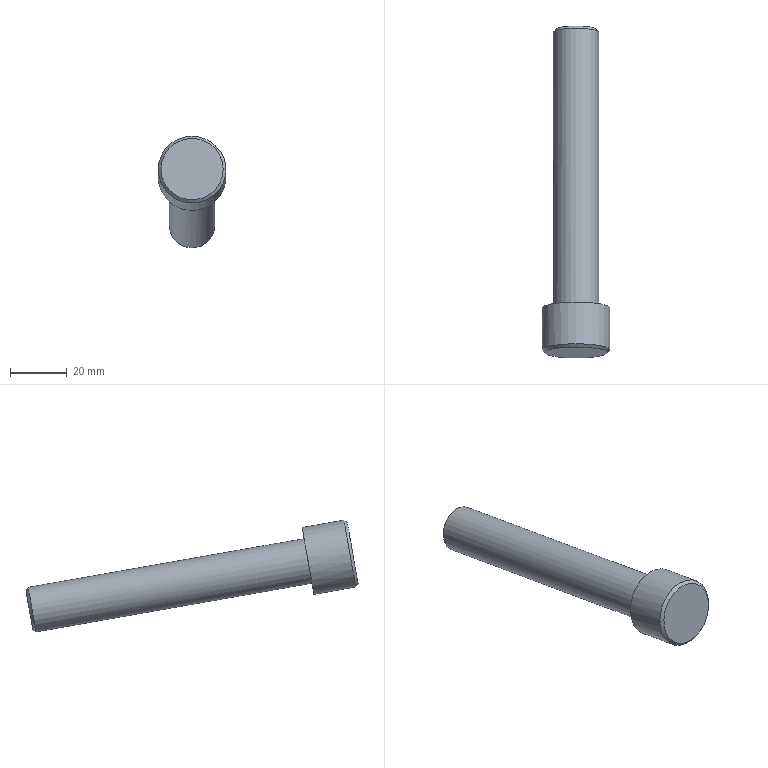Part | NX | features solid 2 | 1 solid | 7 faces | box 24 x 117.363 x 39.492 mm | volume 27284 mm3 | plane 3 | cylinder 2 | cone 2 | commonest cylinder face diameters 16 x1 24 x1
STEP:
#1=CARTESIAN_POINT('',(376.5,-835.707,26.053));
#2=VERTEX_POINT('',#1);
#3=CARTESIAN_POINT('',(376.5,-837.791,14.236));
#4=DIRECTION('',(0.,0.9848,-0.1736));
#5=DIRECTION('',(0.,0.1736,0.9848));
#6=AXIS2_PLACEMENT_3D('',#3,#4,#5);
#7=CIRCLE('',#6,12.);
#8=EDGE_CURVE('',#2,#2,#7,.F.);
#9=ORIENTED_EDGE('',*,*,#8,.F.);
#10=EDGE_LOOP('',(#9));
#11=FACE_BOUND('',#10,.T.);
#12=CARTESIAN_POINT('',(376.5,-836.402,22.114));
#13=VERTEX_POINT('',#12);
#14=CARTESIAN_POINT('',(376.5,-837.791,14.236));
#15=DIRECTION('',(0.,0.9848,-0.1736));
#16=DIRECTION('',(0.,0.1736,0.9848));
#17=AXIS2_PLACEMENT_3D('',#14,#15,#16);
#18=CIRCLE('',#17,8.);
#19=EDGE_CURVE('',#13,#13,#18,.T.);
#20=ORIENTED_EDGE('',*,*,#19,.F.);
#21=EDGE_LOOP('',(#20));
#22=FACE_BOUND('',#21,.T.);
#23=CARTESIAN_POINT('',(376.5,-837.791,14.236));
#24=DIRECTION('',(0.,-0.9848,0.1736));
#25=DIRECTION('',(-1.,0.,0.));
#26=AXIS2_PLACEMENT_3D('',#23,#24,#25);
#27=PLANE('',#26);
#28=ADVANCED_FACE('',(#11,#22),#27,.F.);
#29=CARTESIAN_POINT('',(364.5,-852.563,16.84));
#30=VERTEX_POINT('',#29);
#31=CARTESIAN_POINT('',(376.5,-852.563,16.84));
#32=DIRECTION('',(0.,-0.9848,0.1736));
#33=DIRECTION('',(-1.,0.,0.));
#34=AXIS2_PLACEMENT_3D('',#31,#32,#33);
#35=CIRCLE('',#34,12.);
#36=EDGE_CURVE('',#30,#30,#35,.F.);
#37=ORIENTED_EDGE('',*,*,#36,.T.);
#38=EDGE_LOOP('',(#37));
#39=FACE_BOUND('',#38,.T.);
#40=ORIENTED_EDGE('',*,*,#8,.T.);
#41=EDGE_LOOP('',(#40));
#42=FACE_BOUND('',#41,.T.);
#43=CARTESIAN_POINT('',(376.5,-853.548,17.014));
#44=DIRECTION('',(0.,0.9848,-0.1736));
#45=DIRECTION('',(1.,0.,0.));
#46=AXIS2_PLACEMENT_3D('',#43,#44,#45);
#47=CYLINDRICAL_SURFACE('',#46,12.);
#48=ADVANCED_FACE('',(#39,#42),#47,.T.);
#49=CARTESIAN_POINT('',(365.5,-853.548,17.014));
#50=VERTEX_POINT('',#49);
#51=CARTESIAN_POINT('',(376.5,-853.548,17.014));
#52=DIRECTION('',(0.,-0.9848,0.1736));
#53=DIRECTION('',(-1.,0.,0.));
#54=AXIS2_PLACEMENT_3D('',#51,#52,#53);
#55=CIRCLE('',#54,11.);
#56=EDGE_CURVE('',#50,#50,#55,.T.);
#57=ORIENTED_EDGE('',*,*,#56,.T.);
#58=EDGE_LOOP('',(#57));
#59=FACE_BOUND('',#58,.T.);
#60=CARTESIAN_POINT('',(376.5,-853.548,17.014));
#61=DIRECTION('',(0.,-0.9848,0.1736));
#62=DIRECTION('',(-1.,0.,0.));
#63=AXIS2_PLACEMENT_3D('',#60,#61,#62);
#64=PLANE('',#63);
#65=ADVANCED_FACE('',(#59),#64,.T.);
#66=CARTESIAN_POINT('',(368.5,-740.295,-2.956));
#67=VERTEX_POINT('',#66);
#68=CARTESIAN_POINT('',(376.5,-740.295,-2.956));
#69=DIRECTION('',(0.,-0.9848,0.1736));
#70=DIRECTION('',(-1.,0.,0.));
#71=AXIS2_PLACEMENT_3D('',#68,#69,#70);
#72=CIRCLE('',#71,8.);
#73=EDGE_CURVE('',#67,#67,#72,.T.);
#74=ORIENTED_EDGE('',*,*,#73,.T.);
#75=EDGE_LOOP('',(#74));
#76=FACE_BOUND('',#75,.T.);
#77=ORIENTED_EDGE('',*,*,#19,.T.);
#78=EDGE_LOOP('',(#77));
#79=FACE_BOUND('',#78,.T.);
#80=CARTESIAN_POINT('',(376.5,-916.576,28.127));
#81=DIRECTION('',(0.,0.9848,-0.1736));
#82=DIRECTION('',(1.,0.,0.));
#83=AXIS2_PLACEMENT_3D('',#80,#81,#82);
#84=CYLINDRICAL_SURFACE('',#83,8.);
#85=ADVANCED_FACE('',(#76,#79),#84,.T.);
#86=CARTESIAN_POINT('',(369.5,-739.31,-3.129));
#87=VERTEX_POINT('',#86);
#88=CARTESIAN_POINT('',(376.5,-739.31,-3.129));
#89=DIRECTION('',(0.,-0.9848,0.1736));
#90=DIRECTION('',(-1.,0.,0.));
#91=AXIS2_PLACEMENT_3D('',#88,#89,#90);
#92=CIRCLE('',#91,7.);
#93=EDGE_CURVE('',#87,#87,#92,.F.);
#94=ORIENTED_EDGE('',*,*,#93,.T.);
#95=EDGE_LOOP('',(#94));
#96=FACE_BOUND('',#95,.T.);
#97=CARTESIAN_POINT('',(376.5,-739.31,-3.129));
#98=DIRECTION('',(0.,-0.9848,0.1736));
#99=DIRECTION('',(-1.,0.,0.));
#100=AXIS2_PLACEMENT_3D('',#97,#98,#99);
#101=PLANE('',#100);
#102=ADVANCED_FACE('',(#96),#101,.F.);
#103=ORIENTED_EDGE('',*,*,#93,.F.);
#104=EDGE_LOOP('',(#103));
#105=FACE_BOUND('',#104,.T.);
#106=ORIENTED_EDGE('',*,*,#73,.F.);
#107=EDGE_LOOP('',(#106));
#108=FACE_BOUND('',#107,.T.);
#109=CARTESIAN_POINT('',(376.5,-740.295,-2.956));
#110=DIRECTION('',(0.,-0.9848,0.1736));
#111=DIRECTION('',(-1.,0.,0.));
#112=AXIS2_PLACEMENT_3D('',#109,#110,#111);
#113=CONICAL_SURFACE('',#112,8.,0.7854);
#114=ADVANCED_FACE('',(#105,#108),#113,.T.);
#115=ORIENTED_EDGE('',*,*,#36,.F.);
#116=EDGE_LOOP('',(#115));
#117=FACE_BOUND('',#116,.T.);
#118=ORIENTED_EDGE('',*,*,#56,.F.);
#119=EDGE_LOOP('',(#118));
#120=FACE_BOUND('',#119,.T.);
#121=CARTESIAN_POINT('',(376.5,-853.548,17.014));
#122=DIRECTION('',(0.,0.9848,-0.1736));
#123=DIRECTION('',(1.,0.,0.));
#124=AXIS2_PLACEMENT_3D('',#121,#122,#123);
#125=CONICAL_SURFACE('',#124,11.,0.7854);
#126=ADVANCED_FACE('',(#117,#120),#125,.T.);
#127=CLOSED_SHELL('',(#28,#48,#65,#85,#102,#114,#126));
#128=MANIFOLD_SOLID_BREP('',#127);
#129=(LENGTH_UNIT()NAMED_UNIT(*)SI_UNIT(.MILLI.,.METRE.));
#130=UNCERTAINTY_MEASURE_WITH_UNIT(LENGTH_MEASURE(0.00001),#129,'','');
#131=(NAMED_UNIT(*)PLANE_ANGLE_UNIT()SI_UNIT($,.RADIAN.));
#132=(NAMED_UNIT(*)SI_UNIT($,.STERADIAN.)SOLID_ANGLE_UNIT());
#133=(GEOMETRIC_REPRESENTATION_CONTEXT(3)GLOBAL_UNCERTAINTY_ASSIGNED_CONTEXT((#130))GLOBAL_UNIT_ASSIGNED_CONTEXT((#129,#131,#132))REPRESENTATION_CONTEXT('',''));
#134=ADVANCED_BREP_SHAPE_REPRESENTATION('',(#128),#133);